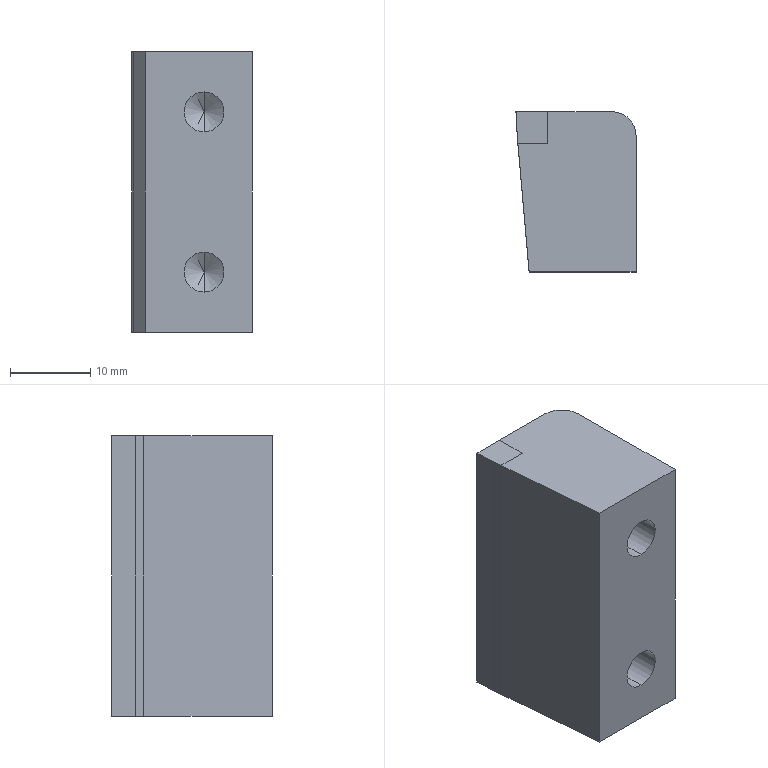Part | SolidWorks | features Extrusion 1, Fillet 1, HoleWzd 1, Split 1 | 2 solids | 24 faces | box 15 x 20 x 35 mm | volume 9279 mm3 | plane 15 | cylinder 5 | cone 4 | commonest cylinder face diameters 5 x4 6 x1
STEP:
#1=CARTESIAN_POINT('',(-11.,20.,-17.5));
#2=VERTEX_POINT('',#1);
#3=CARTESIAN_POINT('',(-11.,20.,17.5));
#4=VERTEX_POINT('',#3);
#5=CARTESIAN_POINT('',(-11.,20.,-17.51));
#6=DIRECTION('',(0.,0.,1.));
#7=VECTOR('',#6,1000.);
#8=LINE('',#5,#7);
#9=EDGE_CURVE('',#2,#4,#8,.T.);
#10=ORIENTED_EDGE('',*,*,#9,.F.);
#11=CARTESIAN_POINT('',(-15.,20.,-17.5));
#12=VERTEX_POINT('',#11);
#13=CARTESIAN_POINT('',(0.,20.,-17.5));
#14=DIRECTION('',(-1.,0.,0.));
#15=VECTOR('',#14,1000.);
#16=LINE('',#13,#15);
#17=EDGE_CURVE('',#2,#12,#16,.T.);
#18=ORIENTED_EDGE('',*,*,#17,.T.);
#19=CARTESIAN_POINT('',(-15.,20.,17.5));
#20=VERTEX_POINT('',#19);
#21=CARTESIAN_POINT('',(-15.,20.,17.5));
#22=DIRECTION('',(0.,0.,-1.));
#23=VECTOR('',#22,1000.);
#24=LINE('',#21,#23);
#25=EDGE_CURVE('',#20,#12,#24,.T.);
#26=ORIENTED_EDGE('',*,*,#25,.F.);
#27=CARTESIAN_POINT('',(0.,20.,17.5));
#28=DIRECTION('',(-1.,0.,0.));
#29=VECTOR('',#28,1000.);
#30=LINE('',#27,#29);
#31=EDGE_CURVE('',#4,#20,#30,.T.);
#32=ORIENTED_EDGE('',*,*,#31,.F.);
#33=EDGE_LOOP('',(#10,#18,#26,#32));
#34=FACE_OUTER_BOUND('',#33,.T.);
#35=CARTESIAN_POINT('',(0.,20.,17.5));
#36=DIRECTION('',(0.,-1.,0.));
#37=DIRECTION('',(1.,0.,0.));
#38=AXIS2_PLACEMENT_3D('',#35,#36,#37);
#39=PLANE('',#38);
#40=ADVANCED_FACE('',(#34),#39,.F.);
#41=CARTESIAN_POINT('',(-14.843,17.,-17.5));
#42=VERTEX_POINT('',#41);
#43=CARTESIAN_POINT('',(-14.843,17.,-17.5));
#44=DIRECTION('',(0.05234,-0.9986,0.));
#45=VECTOR('',#44,1000.);
#46=LINE('',#43,#45);
#47=EDGE_CURVE('',#12,#42,#46,.T.);
#48=ORIENTED_EDGE('',*,*,#47,.T.);
#49=CARTESIAN_POINT('',(-14.843,17.,17.5));
#50=VERTEX_POINT('',#49);
#51=CARTESIAN_POINT('',(-14.843,17.,17.5));
#52=DIRECTION('',(0.,0.,-1.));
#53=VECTOR('',#52,1000.);
#54=LINE('',#51,#53);
#55=EDGE_CURVE('',#50,#42,#54,.T.);
#56=ORIENTED_EDGE('',*,*,#55,.F.);
#57=CARTESIAN_POINT('',(-14.843,17.,17.5));
#58=DIRECTION('',(0.05234,-0.9986,0.));
#59=VECTOR('',#58,1000.);
#60=LINE('',#57,#59);
#61=EDGE_CURVE('',#20,#50,#60,.T.);
#62=ORIENTED_EDGE('',*,*,#61,.F.);
#63=ORIENTED_EDGE('',*,*,#25,.T.);
#64=EDGE_LOOP('',(#48,#56,#62,#63));
#65=FACE_OUTER_BOUND('',#64,.T.);
#66=CARTESIAN_POINT('',(-14.843,17.,17.5));
#67=DIRECTION('',(0.9986,0.05234,0.));
#68=DIRECTION('',(-0.05234,0.9986,0.));
#69=AXIS2_PLACEMENT_3D('',#66,#67,#68);
#70=PLANE('',#69);
#71=ADVANCED_FACE('',(#65),#70,.F.);
#72=CARTESIAN_POINT('',(-14.755,16.,17.5));
#73=VERTEX_POINT('',#72);
#74=CARTESIAN_POINT('',(-14.755,16.,-17.5));
#75=VERTEX_POINT('',#74);
#76=CARTESIAN_POINT('',(-14.755,16.,17.5));
#77=DIRECTION('',(0.,0.,-1.));
#78=VECTOR('',#77,1000.);
#79=LINE('',#76,#78);
#80=EDGE_CURVE('',#73,#75,#79,.T.);
#81=ORIENTED_EDGE('',*,*,#80,.F.);
#82=CARTESIAN_POINT('',(-13.355,0.,17.5));
#83=DIRECTION('',(0.08716,-0.9962,0.));
#84=VECTOR('',#83,1000.);
#85=LINE('',#82,#84);
#86=EDGE_CURVE('',#50,#73,#85,.T.);
#87=ORIENTED_EDGE('',*,*,#86,.F.);
#88=ORIENTED_EDGE('',*,*,#55,.T.);
#89=CARTESIAN_POINT('',(-13.355,0.,-17.5));
#90=DIRECTION('',(0.08716,-0.9962,0.));
#91=VECTOR('',#90,1000.);
#92=LINE('',#89,#91);
#93=EDGE_CURVE('',#42,#75,#92,.T.);
#94=ORIENTED_EDGE('',*,*,#93,.T.);
#95=EDGE_LOOP('',(#81,#87,#88,#94));
#96=FACE_OUTER_BOUND('',#95,.T.);
#97=CARTESIAN_POINT('',(-13.355,0.,17.5));
#98=DIRECTION('',(0.9962,0.08716,0.));
#99=DIRECTION('',(-0.08716,0.9962,0.));
#100=AXIS2_PLACEMENT_3D('',#97,#98,#99);
#101=PLANE('',#100);
#102=ADVANCED_FACE('',(#96),#101,.F.);
#103=CARTESIAN_POINT('',(-11.,16.,-17.5));
#104=VERTEX_POINT('',#103);
#105=CARTESIAN_POINT('',(0.,16.,-17.5));
#106=DIRECTION('',(1.,0.,0.));
#107=VECTOR('',#106,1000.);
#108=LINE('',#105,#107);
#109=EDGE_CURVE('',#75,#104,#108,.T.);
#110=ORIENTED_EDGE('',*,*,#109,.F.);
#111=ORIENTED_EDGE('',*,*,#93,.F.);
#112=ORIENTED_EDGE('',*,*,#47,.F.);
#113=ORIENTED_EDGE('',*,*,#17,.F.);
#114=CARTESIAN_POINT('',(-11.,20.,-17.5));
#115=DIRECTION('',(0.,1.,0.));
#116=VECTOR('',#115,1000.);
#117=LINE('',#114,#116);
#118=EDGE_CURVE('',#104,#2,#117,.T.);
#119=ORIENTED_EDGE('',*,*,#118,.F.);
#120=EDGE_LOOP('',(#110,#111,#112,#113,#119));
#121=FACE_OUTER_BOUND('',#120,.T.);
#122=CARTESIAN_POINT('',(0.,20.,-17.5));
#123=DIRECTION('',(0.,0.,1.));
#124=DIRECTION('',(1.,0.,0.));
#125=AXIS2_PLACEMENT_3D('',#122,#123,#124);
#126=PLANE('',#125);
#127=ADVANCED_FACE('',(#121),#126,.F.);
#128=ORIENTED_EDGE('',*,*,#86,.T.);
#129=CARTESIAN_POINT('',(-11.,16.,17.5));
#130=VERTEX_POINT('',#129);
#131=CARTESIAN_POINT('',(0.,16.,17.5));
#132=DIRECTION('',(1.,0.,0.));
#133=VECTOR('',#132,1000.);
#134=LINE('',#131,#133);
#135=EDGE_CURVE('',#73,#130,#134,.T.);
#136=ORIENTED_EDGE('',*,*,#135,.T.);
#137=CARTESIAN_POINT('',(-11.,20.,17.5));
#138=DIRECTION('',(0.,1.,0.));
#139=VECTOR('',#138,1000.);
#140=LINE('',#137,#139);
#141=EDGE_CURVE('',#130,#4,#140,.T.);
#142=ORIENTED_EDGE('',*,*,#141,.T.);
#143=ORIENTED_EDGE('',*,*,#31,.T.);
#144=ORIENTED_EDGE('',*,*,#61,.T.);
#145=EDGE_LOOP('',(#128,#136,#142,#143,#144));
#146=FACE_OUTER_BOUND('',#145,.T.);
#147=CARTESIAN_POINT('',(0.,20.,17.5));
#148=DIRECTION('',(0.,0.,1.));
#149=DIRECTION('',(1.,0.,0.));
#150=AXIS2_PLACEMENT_3D('',#147,#148,#149);
#151=PLANE('',#150);
#152=ADVANCED_FACE('',(#146),#151,.T.);
#153=CARTESIAN_POINT('',(-11.,16.,-17.51));
#154=DIRECTION('',(0.,0.,1.));
#155=VECTOR('',#154,1000.);
#156=LINE('',#153,#155);
#157=EDGE_CURVE('',#104,#130,#156,.T.);
#158=ORIENTED_EDGE('',*,*,#157,.F.);
#159=ORIENTED_EDGE('',*,*,#118,.T.);
#160=ORIENTED_EDGE('',*,*,#9,.T.);
#161=ORIENTED_EDGE('',*,*,#141,.F.);
#162=EDGE_LOOP('',(#158,#159,#160,#161));
#163=FACE_OUTER_BOUND('',#162,.T.);
#164=CARTESIAN_POINT('',(-11.,20.,-17.51));
#165=DIRECTION('',(1.,0.,0.));
#166=DIRECTION('',(0.,0.,-1.));
#167=AXIS2_PLACEMENT_3D('',#164,#165,#166);
#168=PLANE('',#167);
#169=ADVANCED_FACE('',(#163),#168,.T.);
#170=ORIENTED_EDGE('',*,*,#135,.F.);
#171=ORIENTED_EDGE('',*,*,#80,.T.);
#172=ORIENTED_EDGE('',*,*,#109,.T.);
#173=ORIENTED_EDGE('',*,*,#157,.T.);
#174=EDGE_LOOP('',(#170,#171,#172,#173));
#175=FACE_OUTER_BOUND('',#174,.T.);
#176=CARTESIAN_POINT('',(-15.,16.,-17.51));
#177=DIRECTION('',(0.,-1.,0.));
#178=DIRECTION('',(0.,0.,-1.));
#179=AXIS2_PLACEMENT_3D('',#176,#177,#178);
#180=PLANE('',#179);
#181=ADVANCED_FACE('',(#175),#180,.T.);
#182=CLOSED_SHELL('',(#40,#71,#102,#127,#152,#169,#181));
#183=MANIFOLD_SOLID_BREP('',#182);
#184=CARTESIAN_POINT('',(-6.,15.,12.5));
#185=VERTEX_POINT('',#184);
#186=CARTESIAN_POINT('',(-6.,15.,7.5));
#187=VERTEX_POINT('',#186);
#188=CARTESIAN_POINT('',(-6.,15.,10.));
#189=DIRECTION('',(0.,-1.,0.));
#190=DIRECTION('',(0.,0.,-1.));
#191=AXIS2_PLACEMENT_3D('',#188,#189,#190);
#192=CIRCLE('',#191,2.5);
#193=EDGE_CURVE('',#185,#187,#192,.T.);
#194=ORIENTED_EDGE('',*,*,#193,.F.);
#195=CARTESIAN_POINT('',(-6.,0.,12.5));
#196=VERTEX_POINT('',#195);
#197=CARTESIAN_POINT('',(-6.,0.,12.5));
#198=DIRECTION('',(0.,-1.,0.));
#199=VECTOR('',#198,1000.);
#200=LINE('',#197,#199);
#201=EDGE_CURVE('',#185,#196,#200,.T.);
#202=ORIENTED_EDGE('',*,*,#201,.T.);
#203=CARTESIAN_POINT('',(-6.,0.,7.5));
#204=VERTEX_POINT('',#203);
#205=CARTESIAN_POINT('',(-6.,0.,10.));
#206=DIRECTION('',(0.,-1.,0.));
#207=DIRECTION('',(0.,0.,-1.));
#208=AXIS2_PLACEMENT_3D('',#205,#206,#207);
#209=CIRCLE('',#208,2.5);
#210=EDGE_CURVE('',#196,#204,#209,.T.);
#211=ORIENTED_EDGE('',*,*,#210,.T.);
#212=CARTESIAN_POINT('',(-6.,0.,7.5));
#213=DIRECTION('',(0.,-1.,0.));
#214=VECTOR('',#213,1000.);
#215=LINE('',#212,#214);
#216=EDGE_CURVE('',#187,#204,#215,.T.);
#217=ORIENTED_EDGE('',*,*,#216,.F.);
#218=EDGE_LOOP('',(#194,#202,#211,#217));
#219=FACE_OUTER_BOUND('',#218,.T.);
#220=CARTESIAN_POINT('',(-6.,0.,10.));
#221=DIRECTION('',(0.,-1.,0.));
#222=DIRECTION('',(0.,0.,-1.));
#223=AXIS2_PLACEMENT_3D('',#220,#221,#222);
#224=CYLINDRICAL_SURFACE('',#223,2.5);
#225=ADVANCED_FACE('',(#219),#224,.F.);
#226=CARTESIAN_POINT('',(-6.,16.502,10.));
#227=VERTEX_POINT('',#226);
#228=CARTESIAN_POINT('',(-6.,15.,7.5));
#229=DIRECTION('',(0.,-0.515,-0.8572));
#230=VECTOR('',#229,1000.);
#231=LINE('',#228,#230);
#232=EDGE_CURVE('',#227,#187,#231,.T.);
#233=ORIENTED_EDGE('',*,*,#232,.F.);
#234=CARTESIAN_POINT('',(-6.,15.,12.5));
#235=DIRECTION('',(0.,-0.515,0.8572));
#236=VECTOR('',#235,1000.);
#237=LINE('',#234,#236);
#238=EDGE_CURVE('',#227,#185,#237,.T.);
#239=ORIENTED_EDGE('',*,*,#238,.T.);
#240=ORIENTED_EDGE('',*,*,#193,.T.);
#241=EDGE_LOOP('',(#233,#239,#240));
#242=FACE_OUTER_BOUND('',#241,.T.);
#243=CARTESIAN_POINT('',(-6.,15.,10.));
#244=DIRECTION('',(0.,-1.,0.));
#245=DIRECTION('',(0.,0.,-1.));
#246=AXIS2_PLACEMENT_3D('',#243,#244,#245);
#247=CONICAL_SURFACE('',#246,2.5,1.03);
#248=ADVANCED_FACE('',(#242),#247,.F.);
#249=CARTESIAN_POINT('',(-6.,15.,-7.5));
#250=VERTEX_POINT('',#249);
#251=CARTESIAN_POINT('',(-6.,15.,-12.5));
#252=VERTEX_POINT('',#251);
#253=CARTESIAN_POINT('',(-6.,15.,-10.));
#254=DIRECTION('',(0.,-1.,0.));
#255=DIRECTION('',(0.,0.,-1.));
#256=AXIS2_PLACEMENT_3D('',#253,#254,#255);
#257=CIRCLE('',#256,2.5);
#258=EDGE_CURVE('',#250,#252,#257,.T.);
#259=ORIENTED_EDGE('',*,*,#258,.F.);
#260=CARTESIAN_POINT('',(-6.,0.,-7.5));
#261=VERTEX_POINT('',#260);
#262=CARTESIAN_POINT('',(-6.,0.,-7.5));
#263=DIRECTION('',(0.,-1.,0.));
#264=VECTOR('',#263,1000.);
#265=LINE('',#262,#264);
#266=EDGE_CURVE('',#250,#261,#265,.T.);
#267=ORIENTED_EDGE('',*,*,#266,.T.);
#268=CARTESIAN_POINT('',(-6.,0.,-12.5));
#269=VERTEX_POINT('',#268);
#270=CARTESIAN_POINT('',(-6.,0.,-10.));
#271=DIRECTION('',(0.,-1.,0.));
#272=DIRECTION('',(0.,0.,-1.));
#273=AXIS2_PLACEMENT_3D('',#270,#271,#272);
#274=CIRCLE('',#273,2.5);
#275=EDGE_CURVE('',#261,#269,#274,.T.);
#276=ORIENTED_EDGE('',*,*,#275,.T.);
#277=CARTESIAN_POINT('',(-6.,0.,-12.5));
#278=DIRECTION('',(0.,-1.,0.));
#279=VECTOR('',#278,1000.);
#280=LINE('',#277,#279);
#281=EDGE_CURVE('',#252,#269,#280,.T.);
#282=ORIENTED_EDGE('',*,*,#281,.F.);
#283=EDGE_LOOP('',(#259,#267,#276,#282));
#284=FACE_OUTER_BOUND('',#283,.T.);
#285=CARTESIAN_POINT('',(-6.,0.,-10.));
#286=DIRECTION('',(0.,-1.,0.));
#287=DIRECTION('',(0.,0.,-1.));
#288=AXIS2_PLACEMENT_3D('',#285,#286,#287);
#289=CYLINDRICAL_SURFACE('',#288,2.5);
#290=ADVANCED_FACE('',(#284),#289,.F.);
#291=CARTESIAN_POINT('',(-6.,16.502,-10.));
#292=VERTEX_POINT('',#291);
#293=CARTESIAN_POINT('',(-6.,15.,-12.5));
#294=DIRECTION('',(0.,-0.515,-0.8572));
#295=VECTOR('',#294,1000.);
#296=LINE('',#293,#295);
#297=EDGE_CURVE('',#292,#252,#296,.T.);
#298=ORIENTED_EDGE('',*,*,#297,.F.);
#299=CARTESIAN_POINT('',(-6.,15.,-7.5));
#300=DIRECTION('',(0.,-0.515,0.8572));
#301=VECTOR('',#300,1000.);
#302=LINE('',#299,#301);
#303=EDGE_CURVE('',#292,#250,#302,.T.);
#304=ORIENTED_EDGE('',*,*,#303,.T.);
#305=ORIENTED_EDGE('',*,*,#258,.T.);
#306=EDGE_LOOP('',(#298,#304,#305));
#307=FACE_OUTER_BOUND('',#306,.T.);
#308=CARTESIAN_POINT('',(-6.,15.,-10.));
#309=DIRECTION('',(0.,-1.,0.));
#310=DIRECTION('',(0.,0.,-1.));
#311=AXIS2_PLACEMENT_3D('',#308,#309,#310);
#312=CONICAL_SURFACE('',#311,2.5,1.03);
#313=ADVANCED_FACE('',(#307),#312,.F.);
#314=CARTESIAN_POINT('',(-11.,16.,-17.5));
#315=VERTEX_POINT('',#314);
#316=CARTESIAN_POINT('',(-11.,16.,17.5));
#317=VERTEX_POINT('',#316);
#318=CARTESIAN_POINT('',(-11.,16.,-17.51));
#319=DIRECTION('',(0.,0.,1.));
#320=VECTOR('',#319,1000.);
#321=LINE('',#318,#320);
#322=EDGE_CURVE('',#315,#317,#321,.T.);
#323=ORIENTED_EDGE('',*,*,#322,.T.);
#324=CARTESIAN_POINT('',(-11.,20.,17.5));
#325=VERTEX_POINT('',#324);
#326=CARTESIAN_POINT('',(-11.,20.,17.5));
#327=DIRECTION('',(0.,1.,0.));
#328=VECTOR('',#327,1000.);
#329=LINE('',#326,#328);
#330=EDGE_CURVE('',#317,#325,#329,.T.);
#331=ORIENTED_EDGE('',*,*,#330,.T.);
#332=CARTESIAN_POINT('',(-11.,20.,-17.5));
#333=VERTEX_POINT('',#332);
#334=CARTESIAN_POINT('',(-11.,20.,-17.51));
#335=DIRECTION('',(0.,0.,1.));
#336=VECTOR('',#335,1000.);
#337=LINE('',#334,#336);
#338=EDGE_CURVE('',#333,#325,#337,.T.);
#339=ORIENTED_EDGE('',*,*,#338,.F.);
#340=CARTESIAN_POINT('',(-11.,20.,-17.5));
#341=DIRECTION('',(0.,1.,0.));
#342=VECTOR('',#341,1000.);
#343=LINE('',#340,#342);
#344=EDGE_CURVE('',#315,#333,#343,.T.);
#345=ORIENTED_EDGE('',*,*,#344,.F.);
#346=EDGE_LOOP('',(#323,#331,#339,#345));
#347=FACE_OUTER_BOUND('',#346,.T.);
#348=CARTESIAN_POINT('',(-11.,20.,-17.51));
#349=DIRECTION('',(1.,0.,0.));
#350=DIRECTION('',(0.,0.,-1.));
#351=AXIS2_PLACEMENT_3D('',#348,#349,#350);
#352=PLANE('',#351);
#353=ADVANCED_FACE('',(#347),#352,.F.);
#354=CARTESIAN_POINT('',(-14.755,16.,17.5));
#355=VERTEX_POINT('',#354);
#356=CARTESIAN_POINT('',(0.,16.,17.5));
#357=DIRECTION('',(1.,0.,0.));
#358=VECTOR('',#357,1000.);
#359=LINE('',#356,#358);
#360=EDGE_CURVE('',#355,#317,#359,.T.);
#361=ORIENTED_EDGE('',*,*,#360,.T.);
#362=ORIENTED_EDGE('',*,*,#322,.F.);
#363=CARTESIAN_POINT('',(-14.755,16.,-17.5));
#364=VERTEX_POINT('',#363);
#365=CARTESIAN_POINT('',(0.,16.,-17.5));
#366=DIRECTION('',(1.,0.,0.));
#367=VECTOR('',#366,1000.);
#368=LINE('',#365,#367);
#369=EDGE_CURVE('',#364,#315,#368,.T.);
#370=ORIENTED_EDGE('',*,*,#369,.F.);
#371=CARTESIAN_POINT('',(-14.755,16.,17.5));
#372=DIRECTION('',(0.,0.,-1.));
#373=VECTOR('',#372,1000.);
#374=LINE('',#371,#373);
#375=EDGE_CURVE('',#355,#364,#374,.T.);
#376=ORIENTED_EDGE('',*,*,#375,.F.);
#377=EDGE_LOOP('',(#361,#362,#370,#376));
#378=FACE_OUTER_BOUND('',#377,.T.);
#379=CARTESIAN_POINT('',(-15.,16.,-17.51));
#380=DIRECTION('',(0.,-1.,0.));
#381=DIRECTION('',(0.,0.,-1.));
#382=AXIS2_PLACEMENT_3D('',#379,#380,#381);
#383=PLANE('',#382);
#384=ADVANCED_FACE('',(#378),#383,.F.);
#385=CARTESIAN_POINT('',(-3.,20.,-17.5));
#386=VERTEX_POINT('',#385);
#387=CARTESIAN_POINT('',(0.,20.,-17.5));
#388=DIRECTION('',(-1.,0.,0.));
#389=VECTOR('',#388,1000.);
#390=LINE('',#387,#389);
#391=EDGE_CURVE('',#386,#333,#390,.T.);
#392=ORIENTED_EDGE('',*,*,#391,.F.);
#393=CARTESIAN_POINT('',(0.,17.,-17.5));
#394=VERTEX_POINT('',#393);
#395=CARTESIAN_POINT('',(-3.,17.,-17.5));
#396=DIRECTION('',(0.,0.,-1.));
#397=DIRECTION('',(1.,0.,0.));
#398=AXIS2_PLACEMENT_3D('',#395,#396,#397);
#399=CIRCLE('',#398,3.);
#400=EDGE_CURVE('',#386,#394,#399,.T.);
#401=ORIENTED_EDGE('',*,*,#400,.T.);
#402=CARTESIAN_POINT('',(0.,0.,-17.5));
#403=VERTEX_POINT('',#402);
#404=CARTESIAN_POINT('',(0.,0.,-17.5));
#405=DIRECTION('',(0.,1.,0.));
#406=VECTOR('',#405,1000.);
#407=LINE('',#404,#406);
#408=EDGE_CURVE('',#403,#394,#407,.T.);
#409=ORIENTED_EDGE('',*,*,#408,.F.);
#410=CARTESIAN_POINT('',(-13.355,0.,-17.5));
#411=VERTEX_POINT('',#410);
#412=CARTESIAN_POINT('',(0.,0.,-17.5));
#413=DIRECTION('',(1.,0.,0.));
#414=VECTOR('',#413,1000.);
#415=LINE('',#412,#414);
#416=EDGE_CURVE('',#411,#403,#415,.T.);
#417=ORIENTED_EDGE('',*,*,#416,.F.);
#418=CARTESIAN_POINT('',(-13.355,0.,-17.5));
#419=DIRECTION('',(0.08716,-0.9962,0.));
#420=VECTOR('',#419,1000.);
#421=LINE('',#418,#420);
#422=EDGE_CURVE('',#364,#411,#421,.T.);
#423=ORIENTED_EDGE('',*,*,#422,.F.);
#424=ORIENTED_EDGE('',*,*,#369,.T.);
#425=ORIENTED_EDGE('',*,*,#344,.T.);
#426=EDGE_LOOP('',(#392,#401,#409,#417,#423,#424,#425));
#427=FACE_OUTER_BOUND('',#426,.T.);
#428=CARTESIAN_POINT('',(0.,20.,-17.5));
#429=DIRECTION('',(0.,0.,1.));
#430=DIRECTION('',(1.,0.,0.));
#431=AXIS2_PLACEMENT_3D('',#428,#429,#430);
#432=PLANE('',#431);
#433=ADVANCED_FACE('',(#427),#432,.F.);
#434=CARTESIAN_POINT('',(0.,0.,17.5));
#435=VERTEX_POINT('',#434);
#436=CARTESIAN_POINT('',(0.,17.,17.5));
#437=VERTEX_POINT('',#436);
#438=CARTESIAN_POINT('',(0.,0.,17.5));
#439=DIRECTION('',(0.,1.,0.));
#440=VECTOR('',#439,1000.);
#441=LINE('',#438,#440);
#442=EDGE_CURVE('',#435,#437,#441,.T.);
#443=ORIENTED_EDGE('',*,*,#442,.T.);
#444=CARTESIAN_POINT('',(-3.,20.,17.5));
#445=VERTEX_POINT('',#444);
#446=CARTESIAN_POINT('',(-3.,17.,17.5));
#447=DIRECTION('',(0.,0.,1.));
#448=DIRECTION('',(1.,0.,0.));
#449=AXIS2_PLACEMENT_3D('',#446,#447,#448);
#450=CIRCLE('',#449,3.);
#451=EDGE_CURVE('',#437,#445,#450,.T.);
#452=ORIENTED_EDGE('',*,*,#451,.T.);
#453=CARTESIAN_POINT('',(0.,20.,17.5));
#454=DIRECTION('',(-1.,0.,0.));
#455=VECTOR('',#454,1000.);
#456=LINE('',#453,#455);
#457=EDGE_CURVE('',#445,#325,#456,.T.);
#458=ORIENTED_EDGE('',*,*,#457,.T.);
#459=ORIENTED_EDGE('',*,*,#330,.F.);
#460=ORIENTED_EDGE('',*,*,#360,.F.);
#461=CARTESIAN_POINT('',(-13.355,0.,17.5));
#462=VERTEX_POINT('',#461);
#463=CARTESIAN_POINT('',(-13.355,0.,17.5));
#464=DIRECTION('',(0.08716,-0.9962,0.));
#465=VECTOR('',#464,1000.);
#466=LINE('',#463,#465);
#467=EDGE_CURVE('',#355,#462,#466,.T.);
#468=ORIENTED_EDGE('',*,*,#467,.T.);
#469=CARTESIAN_POINT('',(0.,0.,17.5));
#470=DIRECTION('',(1.,0.,0.));
#471=VECTOR('',#470,1000.);
#472=LINE('',#469,#471);
#473=EDGE_CURVE('',#462,#435,#472,.T.);
#474=ORIENTED_EDGE('',*,*,#473,.T.);
#475=EDGE_LOOP('',(#443,#452,#458,#459,#460,#468,#474));
#476=FACE_OUTER_BOUND('',#475,.T.);
#477=CARTESIAN_POINT('',(0.,20.,17.5));
#478=DIRECTION('',(0.,0.,1.));
#479=DIRECTION('',(1.,0.,0.));
#480=AXIS2_PLACEMENT_3D('',#477,#478,#479);
#481=PLANE('',#480);
#482=ADVANCED_FACE('',(#476),#481,.T.);
#483=CARTESIAN_POINT('',(-6.,0.,10.));
#484=DIRECTION('',(0.,-1.,0.));
#485=DIRECTION('',(0.,0.,-1.));
#486=AXIS2_PLACEMENT_3D('',#483,#484,#485);
#487=CIRCLE('',#486,2.5);
#488=EDGE_CURVE('',#204,#196,#487,.T.);
#489=ORIENTED_EDGE('',*,*,#488,.F.);
#490=ORIENTED_EDGE('',*,*,#210,.F.);
#491=EDGE_LOOP('',(#489,#490));
#492=FACE_BOUND('',#491,.T.);
#493=CARTESIAN_POINT('',(-6.,0.,-10.));
#494=DIRECTION('',(0.,-1.,0.));
#495=DIRECTION('',(0.,0.,-1.));
#496=AXIS2_PLACEMENT_3D('',#493,#494,#495);
#497=CIRCLE('',#496,2.5);
#498=EDGE_CURVE('',#269,#261,#497,.T.);
#499=ORIENTED_EDGE('',*,*,#498,.F.);
#500=ORIENTED_EDGE('',*,*,#275,.F.);
#501=EDGE_LOOP('',(#499,#500));
#502=FACE_BOUND('',#501,.T.);
#503=ORIENTED_EDGE('',*,*,#416,.T.);
#504=CARTESIAN_POINT('',(0.,0.,17.5));
#505=DIRECTION('',(0.,0.,-1.));
#506=VECTOR('',#505,1000.);
#507=LINE('',#504,#506);
#508=EDGE_CURVE('',#435,#403,#507,.T.);
#509=ORIENTED_EDGE('',*,*,#508,.F.);
#510=ORIENTED_EDGE('',*,*,#473,.F.);
#511=CARTESIAN_POINT('',(-13.355,0.,17.5));
#512=DIRECTION('',(0.,0.,-1.));
#513=VECTOR('',#512,1000.);
#514=LINE('',#511,#513);
#515=EDGE_CURVE('',#462,#411,#514,.T.);
#516=ORIENTED_EDGE('',*,*,#515,.T.);
#517=EDGE_LOOP('',(#503,#509,#510,#516));
#518=FACE_OUTER_BOUND('',#517,.T.);
#519=CARTESIAN_POINT('',(0.,0.,17.5));
#520=DIRECTION('',(0.,1.,0.));
#521=DIRECTION('',(-1.,0.,0.));
#522=AXIS2_PLACEMENT_3D('',#519,#520,#521);
#523=PLANE('',#522);
#524=ADVANCED_FACE('',(#492,#502,#518),#523,.F.);
#525=ORIENTED_EDGE('',*,*,#467,.F.);
#526=ORIENTED_EDGE('',*,*,#375,.T.);
#527=ORIENTED_EDGE('',*,*,#422,.T.);
#528=ORIENTED_EDGE('',*,*,#515,.F.);
#529=EDGE_LOOP('',(#525,#526,#527,#528));
#530=FACE_OUTER_BOUND('',#529,.T.);
#531=CARTESIAN_POINT('',(-13.355,0.,17.5));
#532=DIRECTION('',(0.9962,0.08716,0.));
#533=DIRECTION('',(-0.08716,0.9962,0.));
#534=AXIS2_PLACEMENT_3D('',#531,#532,#533);
#535=PLANE('',#534);
#536=ADVANCED_FACE('',(#530),#535,.F.);
#537=ORIENTED_EDGE('',*,*,#457,.F.);
#538=CARTESIAN_POINT('',(-3.,20.,17.5));
#539=DIRECTION('',(0.,0.,-1.));
#540=VECTOR('',#539,1000.);
#541=LINE('',#538,#540);
#542=EDGE_CURVE('',#445,#386,#541,.T.);
#543=ORIENTED_EDGE('',*,*,#542,.T.);
#544=ORIENTED_EDGE('',*,*,#391,.T.);
#545=ORIENTED_EDGE('',*,*,#338,.T.);
#546=EDGE_LOOP('',(#537,#543,#544,#545));
#547=FACE_OUTER_BOUND('',#546,.T.);
#548=CARTESIAN_POINT('',(0.,20.,17.5));
#549=DIRECTION('',(0.,-1.,0.));
#550=DIRECTION('',(1.,0.,0.));
#551=AXIS2_PLACEMENT_3D('',#548,#549,#550);
#552=PLANE('',#551);
#553=ADVANCED_FACE('',(#547),#552,.F.);
#554=ORIENTED_EDGE('',*,*,#408,.T.);
#555=CARTESIAN_POINT('',(0.,17.,17.5));
#556=DIRECTION('',(0.,0.,1.));
#557=VECTOR('',#556,1000.);
#558=LINE('',#555,#557);
#559=EDGE_CURVE('',#394,#437,#558,.T.);
#560=ORIENTED_EDGE('',*,*,#559,.T.);
#561=ORIENTED_EDGE('',*,*,#442,.F.);
#562=ORIENTED_EDGE('',*,*,#508,.T.);
#563=EDGE_LOOP('',(#554,#560,#561,#562));
#564=FACE_OUTER_BOUND('',#563,.T.);
#565=CARTESIAN_POINT('',(0.,0.,17.5));
#566=DIRECTION('',(-1.,0.,0.));
#567=DIRECTION('',(0.,0.,1.));
#568=AXIS2_PLACEMENT_3D('',#565,#566,#567);
#569=PLANE('',#568);
#570=ADVANCED_FACE('',(#564),#569,.F.);
#571=ORIENTED_EDGE('',*,*,#303,.F.);
#572=ORIENTED_EDGE('',*,*,#297,.T.);
#573=CARTESIAN_POINT('',(-6.,15.,-10.));
#574=DIRECTION('',(0.,-1.,0.));
#575=DIRECTION('',(0.,0.,-1.));
#576=AXIS2_PLACEMENT_3D('',#573,#574,#575);
#577=CIRCLE('',#576,2.5);
#578=EDGE_CURVE('',#252,#250,#577,.T.);
#579=ORIENTED_EDGE('',*,*,#578,.T.);
#580=EDGE_LOOP('',(#571,#572,#579));
#581=FACE_OUTER_BOUND('',#580,.T.);
#582=CARTESIAN_POINT('',(-6.,15.,-10.));
#583=DIRECTION('',(0.,-1.,0.));
#584=DIRECTION('',(0.,0.,-1.));
#585=AXIS2_PLACEMENT_3D('',#582,#583,#584);
#586=CONICAL_SURFACE('',#585,2.5,1.03);
#587=ADVANCED_FACE('',(#581),#586,.F.);
#588=ORIENTED_EDGE('',*,*,#266,.F.);
#589=ORIENTED_EDGE('',*,*,#578,.F.);
#590=ORIENTED_EDGE('',*,*,#281,.T.);
#591=ORIENTED_EDGE('',*,*,#498,.T.);
#592=EDGE_LOOP('',(#588,#589,#590,#591));
#593=FACE_OUTER_BOUND('',#592,.T.);
#594=CARTESIAN_POINT('',(-6.,0.,-10.));
#595=DIRECTION('',(0.,-1.,0.));
#596=DIRECTION('',(0.,0.,-1.));
#597=AXIS2_PLACEMENT_3D('',#594,#595,#596);
#598=CYLINDRICAL_SURFACE('',#597,2.5);
#599=ADVANCED_FACE('',(#593),#598,.F.);
#600=ORIENTED_EDGE('',*,*,#238,.F.);
#601=ORIENTED_EDGE('',*,*,#232,.T.);
#602=CARTESIAN_POINT('',(-6.,15.,10.));
#603=DIRECTION('',(0.,-1.,0.));
#604=DIRECTION('',(0.,0.,-1.));
#605=AXIS2_PLACEMENT_3D('',#602,#603,#604);
#606=CIRCLE('',#605,2.5);
#607=EDGE_CURVE('',#187,#185,#606,.T.);
#608=ORIENTED_EDGE('',*,*,#607,.T.);
#609=EDGE_LOOP('',(#600,#601,#608));
#610=FACE_OUTER_BOUND('',#609,.T.);
#611=CARTESIAN_POINT('',(-6.,15.,10.));
#612=DIRECTION('',(0.,-1.,0.));
#613=DIRECTION('',(0.,0.,-1.));
#614=AXIS2_PLACEMENT_3D('',#611,#612,#613);
#615=CONICAL_SURFACE('',#614,2.5,1.03);
#616=ADVANCED_FACE('',(#610),#615,.F.);
#617=ORIENTED_EDGE('',*,*,#201,.F.);
#618=ORIENTED_EDGE('',*,*,#607,.F.);
#619=ORIENTED_EDGE('',*,*,#216,.T.);
#620=ORIENTED_EDGE('',*,*,#488,.T.);
#621=EDGE_LOOP('',(#617,#618,#619,#620));
#622=FACE_OUTER_BOUND('',#621,.T.);
#623=CARTESIAN_POINT('',(-6.,0.,10.));
#624=DIRECTION('',(0.,-1.,0.));
#625=DIRECTION('',(0.,0.,-1.));
#626=AXIS2_PLACEMENT_3D('',#623,#624,#625);
#627=CYLINDRICAL_SURFACE('',#626,2.5);
#628=ADVANCED_FACE('',(#622),#627,.F.);
#629=ORIENTED_EDGE('',*,*,#451,.F.);
#630=ORIENTED_EDGE('',*,*,#559,.F.);
#631=ORIENTED_EDGE('',*,*,#400,.F.);
#632=ORIENTED_EDGE('',*,*,#542,.F.);
#633=EDGE_LOOP('',(#629,#630,#631,#632));
#634=FACE_OUTER_BOUND('',#633,.T.);
#635=CARTESIAN_POINT('',(-3.,17.,17.5));
#636=DIRECTION('',(0.,0.,-1.));
#637=DIRECTION('',(-1.,0.,0.));
#638=AXIS2_PLACEMENT_3D('',#635,#636,#637);
#639=CYLINDRICAL_SURFACE('',#638,3.);
#640=ADVANCED_FACE('',(#634),#639,.T.);
#641=CLOSED_SHELL('',(#225,#248,#290,#313,#353,#384,#433,#482,#524,#536,#553,#570,#587,#599,#616,#628,#640));
#642=MANIFOLD_SOLID_BREP('',#641);
#643=CARTESIAN_POINT('',(0.,0.,0.));
#644=DIRECTION('',(0.,0.,1.));
#645=DIRECTION('',(1.,0.,0.));
#646=AXIS2_PLACEMENT_3D('',#643,#644,#645);
#647=(LENGTH_UNIT()NAMED_UNIT(*)SI_UNIT(.MILLI.,.METRE.));
#648=UNCERTAINTY_MEASURE_WITH_UNIT(LENGTH_MEASURE(0.00001),#647,'','');
#649=(NAMED_UNIT(*)PLANE_ANGLE_UNIT()SI_UNIT($,.RADIAN.));
#650=(NAMED_UNIT(*)SI_UNIT($,.STERADIAN.)SOLID_ANGLE_UNIT());
#651=(GEOMETRIC_REPRESENTATION_CONTEXT(3)GLOBAL_UNCERTAINTY_ASSIGNED_CONTEXT((#648))GLOBAL_UNIT_ASSIGNED_CONTEXT((#647,#649,#650))REPRESENTATION_CONTEXT('',''));
#652=ADVANCED_BREP_SHAPE_REPRESENTATION('',(#183,#642,#646),#651);